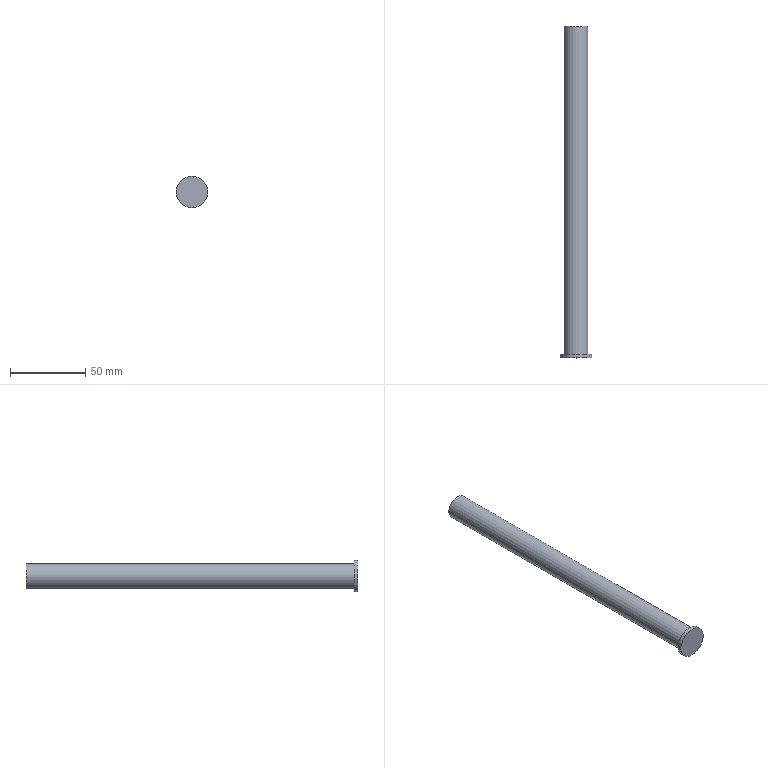Part | STEP file | RETURN-PIN_id302_x_t | 1 solid | 5 faces | box 21 x 221 x 21 mm | volume 44798 mm3 | plane 3 | cylinder 2 | commonest cylinder face diameters 16 x1 21 x1
STEP:
#1=CARTESIAN_POINT('',(-115.,-220.5,-24.5));
#2=VERTEX_POINT('',#1);
#3=CARTESIAN_POINT('',(-115.,-220.5,-35.));
#4=DIRECTION('',(0.,1.,0.));
#5=DIRECTION('',(0.,0.,1.));
#6=AXIS2_PLACEMENT_3D('',#3,#4,#5);
#7=CIRCLE('',#6,10.5);
#8=EDGE_CURVE('',#2,#2,#7,.T.);
#9=ORIENTED_EDGE('',*,*,#8,.F.);
#10=EDGE_LOOP('',(#9));
#11=FACE_OUTER_BOUND('',#10,.T.);
#12=CARTESIAN_POINT('',(-115.,-220.5,-35.));
#13=DIRECTION('',(0.,1.,0.));
#14=DIRECTION('',(0.,0.,1.));
#15=AXIS2_PLACEMENT_3D('',#12,#13,#14);
#16=PLANE('',#15);
#17=ADVANCED_FACE('',(#11),#16,.F.);
#18=ORIENTED_EDGE('',*,*,#8,.T.);
#19=EDGE_LOOP('',(#18));
#20=FACE_BOUND('',#19,.T.);
#21=CARTESIAN_POINT('',(-115.,-218.,-24.5));
#22=VERTEX_POINT('',#21);
#23=CARTESIAN_POINT('',(-115.,-218.,-35.));
#24=DIRECTION('',(0.,1.,0.));
#25=DIRECTION('',(0.,0.,1.));
#26=AXIS2_PLACEMENT_3D('',#23,#24,#25);
#27=CIRCLE('',#26,10.5);
#28=EDGE_CURVE('',#22,#22,#27,.T.);
#29=ORIENTED_EDGE('',*,*,#28,.F.);
#30=EDGE_LOOP('',(#29));
#31=FACE_BOUND('',#30,.T.);
#32=CARTESIAN_POINT('',(-115.,-231.55,-35.));
#33=DIRECTION('',(0.,1.,0.));
#34=DIRECTION('',(0.,0.,1.));
#35=AXIS2_PLACEMENT_3D('',#32,#33,#34);
#36=CYLINDRICAL_SURFACE('',#35,10.5);
#37=ADVANCED_FACE('',(#20,#31),#36,.T.);
#38=CARTESIAN_POINT('',(-115.,0.5,-27.));
#39=VERTEX_POINT('',#38);
#40=CARTESIAN_POINT('',(-115.,0.5,-35.));
#41=DIRECTION('',(0.,-1.,0.));
#42=DIRECTION('',(0.,0.,1.));
#43=AXIS2_PLACEMENT_3D('',#40,#41,#42);
#44=CIRCLE('',#43,8.);
#45=EDGE_CURVE('',#39,#39,#44,.T.);
#46=ORIENTED_EDGE('',*,*,#45,.F.);
#47=EDGE_LOOP('',(#46));
#48=FACE_OUTER_BOUND('',#47,.T.);
#49=CARTESIAN_POINT('',(-115.,0.5,-35.));
#50=DIRECTION('',(0.,1.,0.));
#51=DIRECTION('',(0.,0.,1.));
#52=AXIS2_PLACEMENT_3D('',#49,#50,#51);
#53=PLANE('',#52);
#54=ADVANCED_FACE('',(#48),#53,.T.);
#55=CARTESIAN_POINT('',(-115.,-218.,-27.));
#56=VERTEX_POINT('',#55);
#57=CARTESIAN_POINT('',(-115.,-218.,-35.));
#58=DIRECTION('',(0.,1.,0.));
#59=DIRECTION('',(0.,0.,1.));
#60=AXIS2_PLACEMENT_3D('',#57,#58,#59);
#61=CIRCLE('',#60,8.);
#62=EDGE_CURVE('',#56,#56,#61,.T.);
#63=ORIENTED_EDGE('',*,*,#62,.F.);
#64=EDGE_LOOP('',(#63));
#65=FACE_BOUND('',#64,.T.);
#66=ORIENTED_EDGE('',*,*,#28,.T.);
#67=EDGE_LOOP('',(#66));
#68=FACE_BOUND('',#67,.T.);
#69=CARTESIAN_POINT('',(-115.,-218.,-35.));
#70=DIRECTION('',(0.,1.,0.));
#71=DIRECTION('',(0.,0.,1.));
#72=AXIS2_PLACEMENT_3D('',#69,#70,#71);
#73=PLANE('',#72);
#74=ADVANCED_FACE('',(#65,#68),#73,.T.);
#75=ORIENTED_EDGE('',*,*,#62,.T.);
#76=EDGE_LOOP('',(#75));
#77=FACE_BOUND('',#76,.T.);
#78=ORIENTED_EDGE('',*,*,#45,.T.);
#79=EDGE_LOOP('',(#78));
#80=FACE_BOUND('',#79,.T.);
#81=CARTESIAN_POINT('',(-115.,-231.55,-35.));
#82=DIRECTION('',(0.,1.,0.));
#83=DIRECTION('',(0.,0.,1.));
#84=AXIS2_PLACEMENT_3D('',#81,#82,#83);
#85=CYLINDRICAL_SURFACE('',#84,8.);
#86=ADVANCED_FACE('',(#77,#80),#85,.T.);
#87=CLOSED_SHELL('',(#17,#37,#54,#74,#86));
#88=MANIFOLD_SOLID_BREP('',#87);
#89=(LENGTH_UNIT()NAMED_UNIT(*)SI_UNIT(.MILLI.,.METRE.));
#90=UNCERTAINTY_MEASURE_WITH_UNIT(LENGTH_MEASURE(0.00002),#89,'','');
#91=(NAMED_UNIT(*)PLANE_ANGLE_UNIT()SI_UNIT($,.RADIAN.));
#92=PLANE_ANGLE_MEASURE_WITH_UNIT(PLANE_ANGLE_MEASURE(0.01745),#91);
#93=DIMENSIONAL_EXPONENTS(0.,0.,0.,0.,0.,0.,0.);
#94=(CONVERSION_BASED_UNIT('DEGREE',#92)NAMED_UNIT(#93)PLANE_ANGLE_UNIT());
#95=(NAMED_UNIT(*)SI_UNIT($,.STERADIAN.)SOLID_ANGLE_UNIT());
#96=(GEOMETRIC_REPRESENTATION_CONTEXT(3)GLOBAL_UNCERTAINTY_ASSIGNED_CONTEXT((#90))GLOBAL_UNIT_ASSIGNED_CONTEXT((#89,#94,#95))REPRESENTATION_CONTEXT('',''));
#97=ADVANCED_BREP_SHAPE_REPRESENTATION('',(#88),#96);